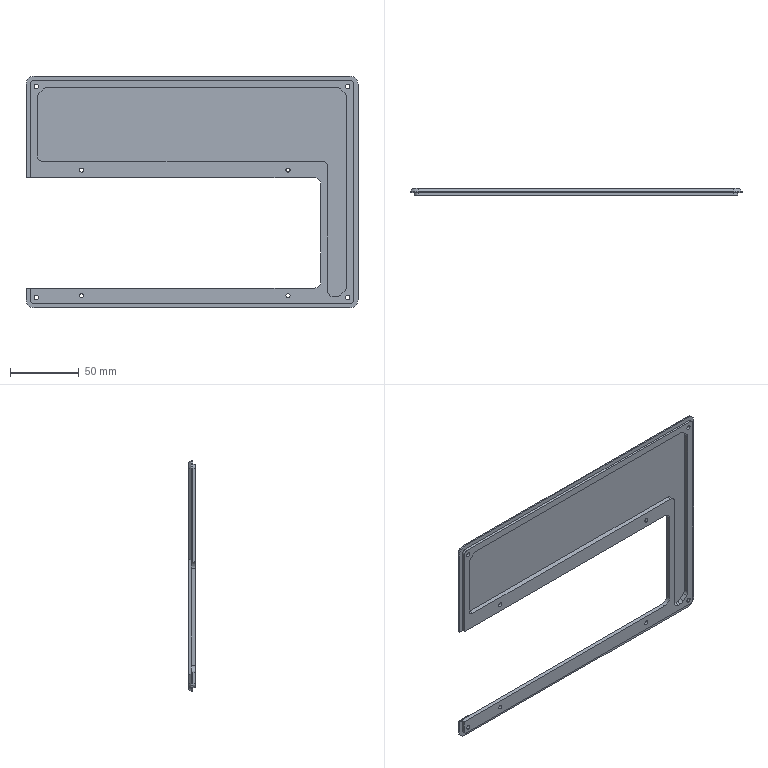NC program | NX | posted by the shop | part box 242 x 5 x 169 mm
Whole program:
%
(CUTTING TIME: 18.83)
(NAME: )
G17 G40 G49 G80 G90
G91 G28 Z0.
(TOOL_NAME :T3-D10-CX )
T03 M06
G00 G90 G54 X123.309 Y90.5 S6500 M03
G43 Z100. H03 M08 T04
G01 X123.309 Y90.5 Z-1.5 F5000.
G41 X123.3 Y90. F1500. D03
X123.3 Y84.5
X123.3 Y-84.5
X123.3 Y-90.
G40 X123.309 Y-90.5
G00 Z50.
G01 X-123.309 Y-90.5 F5000.
X-123.309 Y-90.5 Z-1.5
G41 X-123.3 Y-90. F1500.
X-123.3 Y-84.5
X-123.3 Y84.5
X-123.3 Y90.
G40 X-123.309 Y90.5
G00 Z100.
G00 G90 G54 X126.509 Y90.5 S6500 M03
G01 X126.509 Y90.5 Z-5. F5000.
G41 X126.5 Y90. F1500.
X126.5 Y84.5
X126.5 Y-84.5
X126.5 Y-90.
G40 X126.509 Y-90.5
X126.509 Y90.5 Z-6. F5000.
G41 X126.5 Y90. F1500.
X126.5 Y84.5
X126.5 Y-84.5
X126.5 Y-90.
G40 X126.509 Y-90.5
G00 Z50.
G01 X-126.509 Y-90.5 F5000.
X-126.509 Y-90.5 Z-5.
G41 X-126.5 Y-90. F1500.
X-126.5 Y-84.5
X-126.5 Y84.5
X-126.5 Y90.
G40 X-126.509 Y90.5
X-126.509 Y-90.5 Z-6. F5000.
G41 X-126.5 Y-90. F1500.
X-126.5 Y-84.5
X-126.5 Y84.5
X-126.5 Y90.
G40 X-126.509 Y90.5
G00 Z100.
M05
M09
G91 G28 Z0.
M01
(TOOL_NAME :T4-D10-JX )
T04 M06
G00 G90 G54 X122.809 Y90.5 S6500 M03
G43 Z100. H04 M08 T10
G01 X122.809 Y90.5 Z-2. F5000.
G41 X122.8 Y90. F1500. D04
X122.8 Y84.5
X122.8 Y-84.5
X122.8 Y-90.
G40 X122.809 Y-90.5
G00 Z50.
G01 X-122.809 Y-90.5 F5000.
X-122.809 Y-90.5 Z-2.
G41 X-122.8 Y-90. F1500.
X-122.8 Y-84.5
X-122.8 Y84.5
X-122.8 Y90.
G40 X-122.809 Y90.5
G00 Z100.
G00 G90 G54 X126.009 Y90.5 S6500 M03
G01 X126.009 Y90.5 Z-5. F5000.
G41 X126. Y90. F1500.
X126. Y84.5
X126. Y-84.5
X126. Y-90.
G40 X126.009 Y-90.5
X126.009 Y90.5 Z-6. F5000.
G41 X126. Y90. F1500.
X126. Y84.5
X126. Y-84.5
X126. Y-90.
G40 X126.009 Y-90.5
G00 Z50.
G01 X-126.009 Y-90.5 F5000.
X-126.009 Y-90.5 Z-5.
G41 X-126. Y-90. F1500.
X-126. Y-84.5
X-126. Y84.5
X-126. Y90.
G40 X-126.009 Y90.5
X-126.009 Y-90.5 Z-6. F5000.
G41 X-126. Y-90. F1500.
X-126. Y-84.5
X-126. Y84.5
X-126. Y90.
G40 X-126.009 Y90.5
G00 Z100.
M05
M09
G91 G28 Z0.
M01
(TOOL_NAME :T10-D4-90° )
T10 M06
G00 G90 G54 X118.809 Y87.2 S6500 M03
G43 Z100. H10 M08 T03
G01 X118.809 Y87.2 Z-1. F5000.
G41 X118.8 Y86.7 F500.
X118.8 Y84.5
X118.8 Y-84.5
X118.8 Y-86.7
G40 X118.809 Y-87.2
G00 Z50.
G01 X-118.809 Y-87.2 F5000.
X-118.809 Y-87.2 Z-1.
G41 X-118.8 Y-86.7 F500.
X-118.8 Y-84.5
X-118.8 Y84.5
X-118.8 Y86.7
G40 X-118.809 Y87.2
G00 Z100.
G00 G90 G54 X122.009 Y87.2 S6500 M03
G01 X122.009 Y87.2 Z-3. F5000.
G41 X122. Y86.7 F500.
X122. Y84.5
X122. Y-84.5
X122. Y-86.7
G40 X122.009 Y-87.2
G00 Z48.
G01 X-122.009 Y-87.2 F5000.
X-122.009 Y-87.2 Z-3.
G41 X-122. Y-86.7 F500.
X-122. Y-84.5
X-122. Y84.5
X-122. Y86.7
G40 X-122.009 Y87.2
G00 Z100.
M05
M09
G91 G28 Z0.
M01
M00
M00
(Change clamp)
(TOOL_NAME :T3-D10-CX )
T03 M06
G00 G90 G54 X-128.3 Y73.5 S6500 M03
G43 Z100. H03 M08 T04
G01 X-128.3 Y73.5 Z-1.5 F5000.
G03 X-123.3 Y78.5 I0.0 J5. F1500.
G02 X-115. Y86.8 I8.3 J0.0
G01 X115. Y86.8
G02 X123.3 Y78.5 I0.0 J-8.3
G03 X128.3 Y73.5 I5. J0.0
G00 Z48.5
G01 X128.3 Y-73.5 F5000.
X128.3 Y-73.5 Z-1.5
G03 X123.3 Y-78.5 I0.0 J-5. F1500.
G02 X115. Y-86.8 I-8.3 J0.0
G01 X-115. Y-86.8
G02 X-123.3 Y-78.5 I0.0 J8.3
G03 X-128.3 Y-73.5 I-5. J0.0
G00 Z100.
G00 G90 G54 X127.5 Y-78.009 S6500 M03
G01 X127.5 Y-78.009 Z-6. F5000.
G41 X127. Y-78. F1500. D03
G03 X126.5 Y-78.5 I0.0 J-.5
G02 X115. Y-90. I-11.5 J0.0
G01 X-115. Y-90.
G02 X-126.5 Y-78.5 I0.0 J11.5
G03 X-127. Y-78. I-.5 J0.0
G40 G01 X-127.5 Y-78.009
G00 Z46.5
G01 X-127.5 Y78.009 F5000.
X-127.5 Y78.009 Z-6.
G41 X-127. Y78. F1500.
G03 X-126.5 Y78.5 I0.0 J.5
G02 X-115. Y90. I11.5 J0.0
G01 X115. Y90.
G02 X126.5 Y78.5 I0.0 J-11.5
G03 X127. Y78. I.5 J0.0
G40 G01 X127.5 Y78.009
G00 Z100.
G00 G90 G54 X2.453 Y50.573 S6500 M03
G01 X2.453 Y50.573 Z.5 F5000.
G03 X2.453 Y50.573 Z.006 I-2.453 J-3.773 F100.
X2.453 Y50.573 Z-.487 I-2.453 J-3.773
X2.453 Y50.573 Z-.981 I-2.453 J-3.773
X2.453 Y50.573 Z-1.474 I-2.453 J-3.773
X2.453 Y50.573 Z-1.968 I-2.453 J-3.773
X2.453 Y50.573 Z-2.461 I-2.453 J-3.773
X2.453 Y50.573 Z-2.955 I-2.453 J-3.773
X0.0 Y51.3 Z-3. I-2.453 J-3.773
G01 X-87.8 Y51.3 F2000.
X-87.8 Y47.4
X87.8 Y47.4
X87.8 Y51.3
X0.0 Y51.3
X0.0 Y55.8
X-92.3 Y55.8
X-92.3 Y42.9
X92.3 Y42.9
X92.3 Y55.8
X0.0 Y55.8
X0.0 Y63.3
X-99.8 Y63.3
X-99.8 Y35.4
X95. Y35.4
G02 X99.8 Y34.708 I0.0 J-17.
G01 X99.8 Y63.3
X0.0 Y63.3
X0.0 Y70.8
X-104.865 Y70.8
X-107.3 Y68.365
X-107.3 Y27.9
X95. Y27.9
G02 X104.5 Y18.4 I0.0 J-9.5
G01 X104.5 Y-70.8
X104.865 Y-70.8
X107.3 Y-68.365
X107.3 Y68.365
X104.865 Y70.8
X0.0 Y70.8
X-.2 Y70.8
X-.2 Y70.8 Z0.0
G00 Z100.
M05
M09
G91 G28 Z0.
M01
(TOOL_NAME :T4-D10-JX )
T04 M06
G00 G90 G54 X-127.8 Y73.5 S6500 M03
G43 Z100. H04 M08 T06
G01 X-127.8 Y73.5 Z-2. F5000.
G03 X-122.8 Y78.5 I0.0 J5. F1500.
G02 X-115. Y86.3 I7.8 J0.0
G01 X115. Y86.3
G02 X122.8 Y78.5 I0.0 J-7.8
G03 X127.8 Y73.5 I5. J0.0
G00 Z48.
G01 X127.8 Y-73.5 F5000.
X127.8 Y-73.5 Z-2.
G03 X122.8 Y-78.5 I0.0 J-5. F1500.
G02 X115. Y-86.3 I-7.8 J0.0
G01 X-115. Y-86.3
G02 X-122.8 Y-78.5 I0.0 J7.8
G03 X-127.8 Y-73.5 I-5. J0.0
G00 Z100.
G00 G90 G54 X-131.5 Y73.509 S6500 M03
G01 X-131.5 Y73.509 Z-6. F5000.
G41 X-131. Y73.5 F1500. D04
G03 X-126. Y78.5 I0.0 J5.
G02 X-115. Y89.5 I11. J0.0
G01 X115. Y89.5
G02 X126. Y78.5 I0.0 J-11.
G03 X131. Y73.5 I5. J0.0
G40 G01 X131.5 Y73.509
G00 Z46.5
G01 X131.5 Y-73.509 F5000.
X131.5 Y-73.509 Z-6.
G41 X131. Y-73.5 F1500.
G03 X126. Y-78.5 I0.0 J-5.
G02 X115. Y-89.5 I-11. J0.0
G01 X-115. Y-89.5
G02 X-126. Y-78.5 I0.0 J11.
G03 X-131. Y-73.5 I-5. J0.0
G40 G01 X-131.5 Y-73.509
G00 Z100.
M05
M09
G91 G28 Z0.
M01
(TOOL_NAME :T6-D8-JX )
T06 M06
G00 G90 G54 X2.641 Y51.146 S6500 M03
G43 Z100. H06 M08 T10
G01 X2.641 Y51.146 Z.5 F5000.
G03 X2.641 Y51.146 Z.105 I-2.641 J-2.446 F100.
X2.641 Y51.146 Z-.29 I-2.641 J-2.446
X2.641 Y51.146 Z-.684 I-2.641 J-2.446
X2.641 Y51.146 Z-1.079 I-2.641 J-2.446
X2.641 Y51.146 Z-1.474 I-2.641 J-2.446
X2.641 Y51.146 Z-1.869 I-2.641 J-2.446
X2.641 Y51.146 Z-2.264 I-2.641 J-2.446
X2.641 Y51.146 Z-2.659 I-2.641 J-2.446
X2.641 Y51.146 Z-3.053 I-2.641 J-2.446
X2.641 Y51.146 Z-3.448 I-2.641 J-2.446
X0.0 Y52.3 Z-3.5 I-2.641 J-2.446
G01 X-88.8 Y52.3 F1000.
X-88.8 Y46.4
X88.8 Y46.4
X88.8 Y52.3
X0.0 Y52.3
X0.0 Y56.3
X-92.8 Y56.3
X-92.8 Y42.4
X92.8 Y42.4
X92.8 Y56.3
X0.0 Y56.3
X0.0 Y60.3
X-96.8 Y60.3
X-96.8 Y38.4
X95. Y38.4
G02 X96.8 Y38.319 I0.0 J-20.
G01 X96.8 Y60.3
X0.0 Y60.3
X0.0 Y64.3
X-100.8 Y64.3
X-100.8 Y34.4
X95. Y34.4
G02 X100.8 Y33.312 I0.0 J-16.
G01 X100.8 Y64.3
X0.0 Y64.3
X0.0 Y68.3
X-103.829 Y68.3
X-104.8 Y67.329
X-104.8 Y30.4
X95. Y30.4
G02 X104.8 Y25.325 I0.0 J-12.
G01 X104.8 Y67.329
X103.829 Y68.3
X0.0 Y68.3
X0.0 Y72.3
X-105.486 Y72.3
X-108.8 Y68.986
X-108.8 Y26.4
X95. Y26.4
G02 X103. Y18.4 I0.0 J-8.
G01 X103. Y-72.3
X105.486 Y-72.3
X108.8 Y-68.986
X108.8 Y68.986
X105.486 Y72.3
X0.0 Y72.3
X-.2 Y72.3
X-.2 Y72.3 Z-.5
G00 Z100.
M05
M09
G91 G28 Z0.
M01
(TOOL_NAME :T10-D4-90° )
T10 M06
G00 G90 G54 X124.3 Y-73.509 S6500 M03
G43 Z100. H10 M08 T12
G01 X124.3 Y-73.509 Z-1. F5000.
G41 X123.8 Y-73.5 F500.
G03 X118.8 Y-78.5 I0.0 J-5.
G02 X115. Y-82.3 I-3.8 J0.0
G01 X-115. Y-82.3
G02 X-118.8 Y-78.5 I0.0 J3.8
G03 X-123.8 Y-73.5 I-5. J0.0
G40 G01 X-124.3 Y-73.509
G00 Z50.
G01 X-124.3 Y73.509 F5000.
X-124.3 Y73.509 Z-1.
G41 X-123.8 Y73.5 F500.
G03 X-118.8 Y78.5 I0.0 J5.
G02 X-115. Y82.3 I3.8 J0.0
G01 X115. Y82.3
G02 X118.8 Y78.5 I0.0 J-3.8
G03 X123.8 Y73.5 I5. J0.0
G40 G01 X124.3 Y73.509
G00 Z100.
G00 G90 G54 X-127.5 Y73.509 S6500 M03
G01 X-127.5 Y73.509 Z-3. F5000.
G41 X-127. Y73.5 F500.
G03 X-122. Y78.5 I0.0 J5.
G02 X-115. Y85.5 I7. J0.0
G01 X115. Y85.5
G02 X122. Y78.5 I0.0 J-7.
G03 X127. Y73.5 I5. J0.0
G40 G01 X127.5 Y73.509
G00 Z48.
G01 X127.5 Y-73.509 F5000.
X127.5 Y-73.509 Z-3.
G41 X127. Y-73.5 F500.
G03 X122. Y-78.5 I0.0 J-5.
G02 X115. Y-85.5 I-7. J0.0
G01 X-115. Y-85.5
G02 X-122. Y-78.5 I0.0 J7.
G03 X-127. Y-73.5 I-5. J0.0
G40 G01 X-127.5 Y-73.509
G00 Z100.
G00 G90 G54 X4.991 Y69.8 S6500 M03
G01 X4.991 Y69.8 Z-1. F5000.
G41 X5. Y70.3 F500.
G03 X0.0 Y75.3 I-5. J0.0
G01 X-105.486 Y75.3
G03 X-107.608 Y74.421 I0.0 J-3.
G01 X-110.921 Y71.108
G03 X-111.8 Y68.986 I2.121 J-2.121
G01 X-111.8 Y26.4
G03 X-108.8 Y23.4 I3. J0.0
G01 X95. Y23.4
G02 X100. Y18.4 I0.0 J-5.
G01 X100. Y-72.3
G03 X103. Y-75.3 I3. J0.0
G01 X105.486 Y-75.3
G03 X107.608 Y-74.421 I0.0 J3.
G01 X110.921 Y-71.108
G03 X111.8 Y-68.986 I-2.121 J2.121
G01 X111.8 Y68.986
G03 X110.921 Y71.108 I-3. J0.0
G01 X107.608 Y74.421
G03 X105.486 Y75.3 I-2.121 J-2.121
G01 X0.0 Y75.3
X-.2 Y75.3
G03 X-5.2 Y70.3 I0.0 J-5.
G40 G01 X-5.191 Y69.8
G00 Z100.
G00 G90 G54 X-113.5 Y77. S1200 M03
Z50.
G98 G83 X-113.5 Y77. Z-.5 R1.5 F100. Q2.
X113.5 Y77.
X113.5 Y-77.
X-113.5 Y-77.
G80
G00 Z50.
G00 G90 G54 X-80.5 Y15.95 S1200 M03
G98 G83 X-80.5 Y15.95 Z-.5 R1.5 F100. Q2.
X70. Y15.95
X-80.5 Y-75.55
X70. Y-75.55
G80
G00 Z50.
M05
M09
G91 G28 Z0.
M01
(TOOL_NAME :T12-ZT3.2 )
T12 M06
G00 G90 G54 X-113.5 Y77. S1200 M03
G43 Z50. H12 M08 T14
G98 G83 X-113.5 Y77. Z-7. R1.5 F100. Q2.
X113.5 Y77.
X113.5 Y-77.
X-113.5 Y-77.
G80
G00 Z50.
M05
M09
G91 G28 Z0.
M01
(TOOL_NAME :T14-ZT2.75 )
T14 M06
G00 G90 G54 X-80.5 Y15.95 S1200 M03
G43 Z50. H14 M08 T15
G98 G83 X-80.5 Y15.95 Z-7. R1.5 F100. Q2.
X70. Y15.95
X-80.5 Y-75.55
X70. Y-75.55
G80
G00 Z50.
M05
M09
G91 G28 Z0.
M01
(TOOL_NAME :T15-M3 )
T15 M06
G00 G90 G54 X-80.5 Y15.95 S1200 M03
G43 Z50. H15 M08 T03
G98 G83 X-80.5 Y15.95 Z-6. R1.5 F100. Q2.
X70. Y15.95
X-80.5 Y-75.55
X70. Y-75.55
G80
G00 Z50.
M05
M09
G91 G28 Z0.
G91 G28 Y0.
M30
%